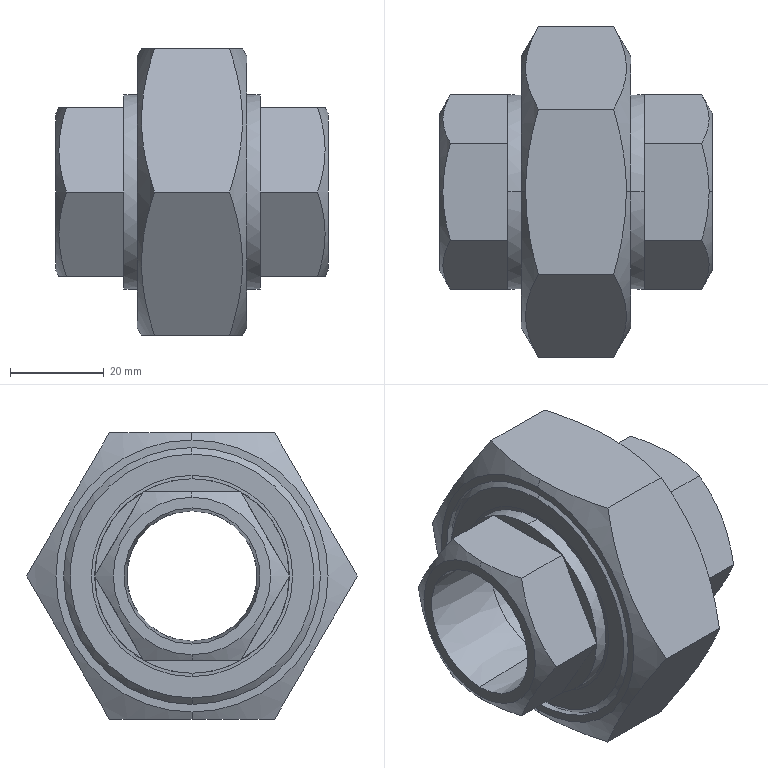Part | SolidWorks | features Cut 4, Revolution 3, Chamfer 1, MirrorPattern 1 | 1 solid | 66 faces | box 58 x 70.38 x 60.951 mm | volume 76848 mm3 | plane 36 | cone 16 | cylinder 10 | torus 4 | commonest cylinder face diameters 41.4 x4 27.74 x2 47.61 x2 54.648 x2